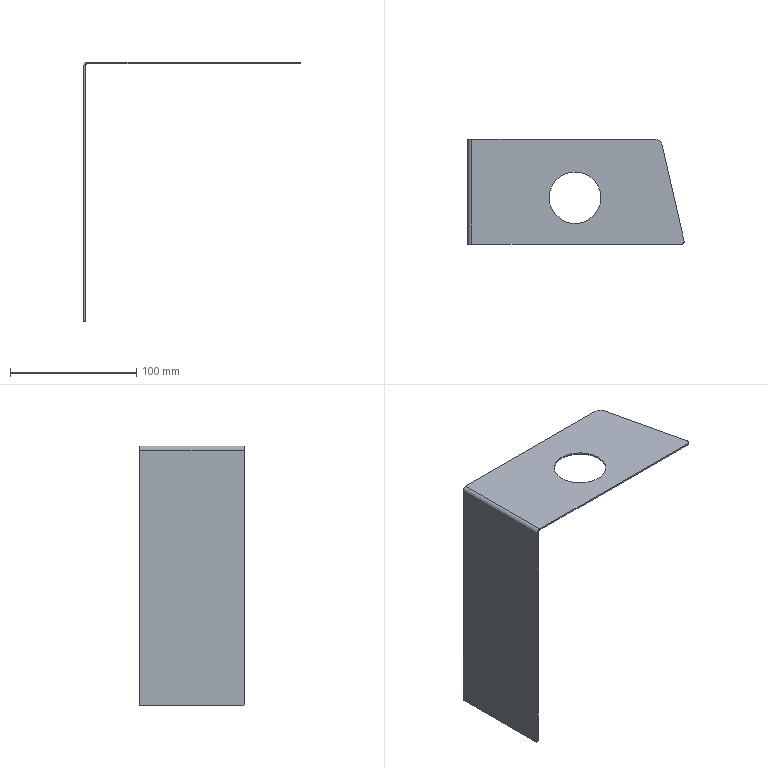Part | SolidWorks | features Fillet 2, FlatPattern 1, ICE 1, SMBaseFlange 1, SheetMetal 1 | 1 solid | 20 faces | box 171.49 x 83 x 206 mm | volume 34881 mm3 | plane 12 | cylinder 8 | commonest cylinder face diameters 4 x4 41 x2 6.4 x1 10 x1
STEP:
#1=CARTESIAN_POINT('',(171.49,2.,204.8));
#2=VERTEX_POINT('',#1);
#3=CARTESIAN_POINT('',(169.49,0.,204.8));
#4=VERTEX_POINT('',#3);
#5=CARTESIAN_POINT('',(169.49,2.,204.8));
#6=DIRECTION('',(0.,0.,-1.));
#7=DIRECTION('',(-1.,0.,0.));
#8=AXIS2_PLACEMENT_3D('',#5,#6,#7);
#9=CIRCLE('',#8,2.);
#10=EDGE_CURVE('',#2,#4,#9,.T.);
#11=ORIENTED_EDGE('',*,*,#10,.F.);
#12=CARTESIAN_POINT('',(171.49,2.,206.));
#13=VERTEX_POINT('',#12);
#14=CARTESIAN_POINT('',(171.49,2.,202.8));
#15=DIRECTION('',(0.,0.,1.));
#16=VECTOR('',#15,1000.);
#17=LINE('',#14,#16);
#18=EDGE_CURVE('',#2,#13,#17,.T.);
#19=ORIENTED_EDGE('',*,*,#18,.T.);
#20=CARTESIAN_POINT('',(169.49,0.,206.));
#21=VERTEX_POINT('',#20);
#22=CARTESIAN_POINT('',(169.49,2.,206.));
#23=DIRECTION('',(0.,0.,1.));
#24=DIRECTION('',(-1.,0.,0.));
#25=AXIS2_PLACEMENT_3D('',#22,#23,#24);
#26=CIRCLE('',#25,2.);
#27=EDGE_CURVE('',#21,#13,#26,.T.);
#28=ORIENTED_EDGE('',*,*,#27,.F.);
#29=CARTESIAN_POINT('',(169.49,0.,202.8));
#30=DIRECTION('',(0.,0.,1.));
#31=VECTOR('',#30,1000.);
#32=LINE('',#29,#31);
#33=EDGE_CURVE('',#4,#21,#32,.T.);
#34=ORIENTED_EDGE('',*,*,#33,.F.);
#35=EDGE_LOOP('',(#11,#19,#28,#34));
#36=FACE_OUTER_BOUND('',#35,.T.);
#37=CARTESIAN_POINT('',(169.49,2.,202.8));
#38=DIRECTION('',(0.,0.,1.));
#39=DIRECTION('',(1.,0.,0.));
#40=AXIS2_PLACEMENT_3D('',#37,#38,#39);
#41=CYLINDRICAL_SURFACE('',#40,2.);
#42=ADVANCED_FACE('',(#36),#41,.T.);
#43=CARTESIAN_POINT('',(64.5,36.8,206.));
#44=VERTEX_POINT('',#43);
#45=CARTESIAN_POINT('',(105.5,36.8,206.));
#46=VERTEX_POINT('',#45);
#47=CARTESIAN_POINT('',(85.,36.8,206.));
#48=DIRECTION('',(0.,0.,1.));
#49=DIRECTION('',(-1.,0.,0.));
#50=AXIS2_PLACEMENT_3D('',#47,#48,#49);
#51=CIRCLE('',#50,20.5);
#52=EDGE_CURVE('',#44,#46,#51,.T.);
#53=ORIENTED_EDGE('',*,*,#52,.T.);
#54=CARTESIAN_POINT('',(105.5,36.8,204.8));
#55=VERTEX_POINT('',#54);
#56=CARTESIAN_POINT('',(105.5,36.8,204.8));
#57=DIRECTION('',(0.,0.,-1.));
#58=VECTOR('',#57,1000.);
#59=LINE('',#56,#58);
#60=EDGE_CURVE('',#46,#55,#59,.T.);
#61=ORIENTED_EDGE('',*,*,#60,.T.);
#62=CARTESIAN_POINT('',(64.5,36.8,204.8));
#63=VERTEX_POINT('',#62);
#64=CARTESIAN_POINT('',(85.,36.8,204.8));
#65=DIRECTION('',(0.,0.,1.));
#66=DIRECTION('',(-1.,0.,0.));
#67=AXIS2_PLACEMENT_3D('',#64,#65,#66);
#68=CIRCLE('',#67,20.5);
#69=EDGE_CURVE('',#63,#55,#68,.T.);
#70=ORIENTED_EDGE('',*,*,#69,.F.);
#71=CARTESIAN_POINT('',(64.5,36.8,204.8));
#72=DIRECTION('',(0.,0.,-1.));
#73=VECTOR('',#72,1000.);
#74=LINE('',#71,#73);
#75=EDGE_CURVE('',#44,#63,#74,.T.);
#76=ORIENTED_EDGE('',*,*,#75,.F.);
#77=EDGE_LOOP('',(#53,#61,#70,#76));
#78=FACE_OUTER_BOUND('',#77,.T.);
#79=CARTESIAN_POINT('',(85.,36.8,204.8));
#80=DIRECTION('',(0.,0.,-1.));
#81=DIRECTION('',(-1.,0.,0.));
#82=AXIS2_PLACEMENT_3D('',#79,#80,#81);
#83=CYLINDRICAL_SURFACE('',#82,20.5);
#84=ADVANCED_FACE('',(#78),#83,.F.);
#85=CARTESIAN_POINT('',(3.2,0.,206.));
#86=VERTEX_POINT('',#85);
#87=CARTESIAN_POINT('',(0.,0.,206.));
#88=DIRECTION('',(1.,0.,0.));
#89=VECTOR('',#88,1000.);
#90=LINE('',#87,#89);
#91=EDGE_CURVE('',#86,#21,#90,.T.);
#92=ORIENTED_EDGE('',*,*,#91,.T.);
#93=ORIENTED_EDGE('',*,*,#27,.T.);
#94=CARTESIAN_POINT('',(171.44,2.446,206.));
#95=VERTEX_POINT('',#94);
#96=CARTESIAN_POINT('',(169.49,2.,206.));
#97=DIRECTION('',(0.,0.,1.));
#98=DIRECTION('',(-1.,0.,0.));
#99=AXIS2_PLACEMENT_3D('',#96,#97,#98);
#100=CIRCLE('',#99,2.);
#101=EDGE_CURVE('',#13,#95,#100,.T.);
#102=ORIENTED_EDGE('',*,*,#101,.T.);
#103=CARTESIAN_POINT('',(153.889,79.116,206.));
#104=VERTEX_POINT('',#103);
#105=CARTESIAN_POINT('',(153.,83.,206.));
#106=DIRECTION('',(0.2231,-0.9748,0.));
#107=VECTOR('',#106,1000.);
#108=LINE('',#105,#107);
#109=EDGE_CURVE('',#104,#95,#108,.T.);
#110=ORIENTED_EDGE('',*,*,#109,.F.);
#111=CARTESIAN_POINT('',(149.015,83.,206.));
#112=VERTEX_POINT('',#111);
#113=CARTESIAN_POINT('',(149.015,78.,206.));
#114=DIRECTION('',(0.,0.,1.));
#115=DIRECTION('',(-1.,0.,0.));
#116=AXIS2_PLACEMENT_3D('',#113,#114,#115);
#117=CIRCLE('',#116,5.);
#118=EDGE_CURVE('',#104,#112,#117,.T.);
#119=ORIENTED_EDGE('',*,*,#118,.T.);
#120=CARTESIAN_POINT('',(3.2,83.,206.));
#121=VERTEX_POINT('',#120);
#122=CARTESIAN_POINT('',(0.,83.,206.));
#123=DIRECTION('',(1.,0.,0.));
#124=VECTOR('',#123,1000.);
#125=LINE('',#122,#124);
#126=EDGE_CURVE('',#121,#112,#125,.T.);
#127=ORIENTED_EDGE('',*,*,#126,.F.);
#128=CARTESIAN_POINT('',(3.2,83.,206.));
#129=DIRECTION('',(0.,-1.,0.));
#130=VECTOR('',#129,1000.);
#131=LINE('',#128,#130);
#132=EDGE_CURVE('',#121,#86,#131,.T.);
#133=ORIENTED_EDGE('',*,*,#132,.T.);
#134=EDGE_LOOP('',(#92,#93,#102,#110,#119,#127,#133));
#135=FACE_OUTER_BOUND('',#134,.T.);
#136=ORIENTED_EDGE('',*,*,#52,.F.);
#137=CARTESIAN_POINT('',(85.,36.8,206.));
#138=DIRECTION('',(0.,0.,1.));
#139=DIRECTION('',(-1.,0.,0.));
#140=AXIS2_PLACEMENT_3D('',#137,#138,#139);
#141=CIRCLE('',#140,20.5);
#142=EDGE_CURVE('',#46,#44,#141,.T.);
#143=ORIENTED_EDGE('',*,*,#142,.F.);
#144=EDGE_LOOP('',(#136,#143));
#145=FACE_BOUND('',#144,.T.);
#146=CARTESIAN_POINT('',(0.,83.,206.));
#147=DIRECTION('',(0.,0.,-1.));
#148=DIRECTION('',(-1.,0.,0.));
#149=AXIS2_PLACEMENT_3D('',#146,#147,#148);
#150=PLANE('',#149);
#151=ADVANCED_FACE('',(#135,#145),#150,.F.);
#152=CARTESIAN_POINT('',(153.889,79.116,204.8));
#153=VERTEX_POINT('',#152);
#154=CARTESIAN_POINT('',(171.44,2.446,204.8));
#155=VERTEX_POINT('',#154);
#156=CARTESIAN_POINT('',(153.,83.,204.8));
#157=DIRECTION('',(0.2231,-0.9748,0.));
#158=VECTOR('',#157,1000.);
#159=LINE('',#156,#158);
#160=EDGE_CURVE('',#153,#155,#159,.T.);
#161=ORIENTED_EDGE('',*,*,#160,.T.);
#162=CARTESIAN_POINT('',(169.49,2.,204.8));
#163=DIRECTION('',(0.,0.,-1.));
#164=DIRECTION('',(-1.,0.,0.));
#165=AXIS2_PLACEMENT_3D('',#162,#163,#164);
#166=CIRCLE('',#165,2.);
#167=EDGE_CURVE('',#155,#2,#166,.T.);
#168=ORIENTED_EDGE('',*,*,#167,.T.);
#169=ORIENTED_EDGE('',*,*,#10,.T.);
#170=CARTESIAN_POINT('',(3.2,0.,204.8));
#171=VERTEX_POINT('',#170);
#172=CARTESIAN_POINT('',(0.,0.,204.8));
#173=DIRECTION('',(1.,0.,0.));
#174=VECTOR('',#173,1000.);
#175=LINE('',#172,#174);
#176=EDGE_CURVE('',#171,#4,#175,.T.);
#177=ORIENTED_EDGE('',*,*,#176,.F.);
#178=CARTESIAN_POINT('',(3.2,83.,204.8));
#179=VERTEX_POINT('',#178);
#180=CARTESIAN_POINT('',(3.2,83.,204.8));
#181=DIRECTION('',(0.,-1.,0.));
#182=VECTOR('',#181,1000.);
#183=LINE('',#180,#182);
#184=EDGE_CURVE('',#179,#171,#183,.T.);
#185=ORIENTED_EDGE('',*,*,#184,.F.);
#186=CARTESIAN_POINT('',(149.015,83.,204.8));
#187=VERTEX_POINT('',#186);
#188=CARTESIAN_POINT('',(0.,83.,204.8));
#189=DIRECTION('',(1.,0.,0.));
#190=VECTOR('',#189,1000.);
#191=LINE('',#188,#190);
#192=EDGE_CURVE('',#179,#187,#191,.T.);
#193=ORIENTED_EDGE('',*,*,#192,.T.);
#194=CARTESIAN_POINT('',(149.015,78.,204.8));
#195=DIRECTION('',(0.,0.,-1.));
#196=DIRECTION('',(-1.,0.,0.));
#197=AXIS2_PLACEMENT_3D('',#194,#195,#196);
#198=CIRCLE('',#197,5.);
#199=EDGE_CURVE('',#187,#153,#198,.T.);
#200=ORIENTED_EDGE('',*,*,#199,.T.);
#201=EDGE_LOOP('',(#161,#168,#169,#177,#185,#193,#200));
#202=FACE_OUTER_BOUND('',#201,.T.);
#203=ORIENTED_EDGE('',*,*,#69,.T.);
#204=CARTESIAN_POINT('',(85.,36.8,204.8));
#205=DIRECTION('',(0.,0.,1.));
#206=DIRECTION('',(-1.,0.,0.));
#207=AXIS2_PLACEMENT_3D('',#204,#205,#206);
#208=CIRCLE('',#207,20.5);
#209=EDGE_CURVE('',#55,#63,#208,.T.);
#210=ORIENTED_EDGE('',*,*,#209,.T.);
#211=EDGE_LOOP('',(#203,#210));
#212=FACE_BOUND('',#211,.T.);
#213=CARTESIAN_POINT('',(0.,83.,204.8));
#214=DIRECTION('',(0.,0.,-1.));
#215=DIRECTION('',(-1.,0.,0.));
#216=AXIS2_PLACEMENT_3D('',#213,#214,#215);
#217=PLANE('',#216);
#218=ADVANCED_FACE('',(#202,#212),#217,.T.);
#219=ORIENTED_EDGE('',*,*,#126,.T.);
#220=CARTESIAN_POINT('',(149.015,83.,202.8));
#221=DIRECTION('',(0.,0.,-1.));
#222=VECTOR('',#221,1000.);
#223=LINE('',#220,#222);
#224=EDGE_CURVE('',#112,#187,#223,.T.);
#225=ORIENTED_EDGE('',*,*,#224,.T.);
#226=ORIENTED_EDGE('',*,*,#192,.F.);
#227=CARTESIAN_POINT('',(3.2,83.,204.8));
#228=DIRECTION('',(0.,0.,1.));
#229=VECTOR('',#228,1000.);
#230=LINE('',#227,#229);
#231=EDGE_CURVE('',#179,#121,#230,.T.);
#232=ORIENTED_EDGE('',*,*,#231,.T.);
#233=EDGE_LOOP('',(#219,#225,#226,#232));
#234=FACE_OUTER_BOUND('',#233,.T.);
#235=CARTESIAN_POINT('',(3.2,83.,202.8));
#236=DIRECTION('',(0.,1.,0.));
#237=DIRECTION('',(1.,0.,0.));
#238=AXIS2_PLACEMENT_3D('',#235,#236,#237);
#239=PLANE('',#238);
#240=ADVANCED_FACE('',(#234),#239,.T.);
#241=CARTESIAN_POINT('',(0.,83.,202.8));
#242=VERTEX_POINT('',#241);
#243=CARTESIAN_POINT('',(1.2,83.,202.8));
#244=VERTEX_POINT('',#243);
#245=CARTESIAN_POINT('',(0.,83.,202.8));
#246=DIRECTION('',(1.,0.,0.));
#247=VECTOR('',#246,1000.);
#248=LINE('',#245,#247);
#249=EDGE_CURVE('',#242,#244,#248,.T.);
#250=ORIENTED_EDGE('',*,*,#249,.F.);
#251=CARTESIAN_POINT('',(3.2,83.,202.8));
#252=DIRECTION('',(0.,1.,0.));
#253=DIRECTION('',(0.,0.,-1.));
#254=AXIS2_PLACEMENT_3D('',#251,#252,#253);
#255=CIRCLE('',#254,3.2);
#256=EDGE_CURVE('',#242,#121,#255,.T.);
#257=ORIENTED_EDGE('',*,*,#256,.T.);
#258=ORIENTED_EDGE('',*,*,#231,.F.);
#259=CARTESIAN_POINT('',(3.2,83.,202.8));
#260=DIRECTION('',(0.,1.,0.));
#261=DIRECTION('',(1.,0.,0.));
#262=AXIS2_PLACEMENT_3D('',#259,#260,#261);
#263=CIRCLE('',#262,2.);
#264=EDGE_CURVE('',#244,#179,#263,.T.);
#265=ORIENTED_EDGE('',*,*,#264,.F.);
#266=EDGE_LOOP('',(#250,#257,#258,#265));
#267=FACE_OUTER_BOUND('',#266,.T.);
#268=CARTESIAN_POINT('',(0.,83.,202.8));
#269=DIRECTION('',(0.,1.,0.));
#270=DIRECTION('',(0.,0.,1.));
#271=AXIS2_PLACEMENT_3D('',#268,#269,#270);
#272=PLANE('',#271);
#273=ADVANCED_FACE('',(#267),#272,.T.);
#274=CARTESIAN_POINT('',(0.,83.,0.));
#275=VERTEX_POINT('',#274);
#276=CARTESIAN_POINT('',(0.,83.,0.));
#277=DIRECTION('',(0.,0.,1.));
#278=VECTOR('',#277,1000.);
#279=LINE('',#276,#278);
#280=EDGE_CURVE('',#275,#242,#279,.T.);
#281=ORIENTED_EDGE('',*,*,#280,.T.);
#282=ORIENTED_EDGE('',*,*,#249,.T.);
#283=CARTESIAN_POINT('',(1.2,83.,0.));
#284=VERTEX_POINT('',#283);
#285=CARTESIAN_POINT('',(1.2,83.,0.));
#286=DIRECTION('',(0.,0.,1.));
#287=VECTOR('',#286,1000.);
#288=LINE('',#285,#287);
#289=EDGE_CURVE('',#284,#244,#288,.T.);
#290=ORIENTED_EDGE('',*,*,#289,.F.);
#291=CARTESIAN_POINT('',(0.,83.,0.));
#292=DIRECTION('',(1.,0.,0.));
#293=VECTOR('',#292,1000.);
#294=LINE('',#291,#293);
#295=EDGE_CURVE('',#275,#284,#294,.T.);
#296=ORIENTED_EDGE('',*,*,#295,.F.);
#297=EDGE_LOOP('',(#281,#282,#290,#296));
#298=FACE_OUTER_BOUND('',#297,.T.);
#299=CARTESIAN_POINT('',(3.2,83.,204.8));
#300=DIRECTION('',(0.,1.,0.));
#301=DIRECTION('',(0.,0.,1.));
#302=AXIS2_PLACEMENT_3D('',#299,#300,#301);
#303=PLANE('',#302);
#304=ADVANCED_FACE('',(#298),#303,.T.);
#305=CARTESIAN_POINT('',(3.2,0.,206.));
#306=DIRECTION('',(0.,0.,-1.));
#307=VECTOR('',#306,1000.);
#308=LINE('',#305,#307);
#309=EDGE_CURVE('',#86,#171,#308,.T.);
#310=ORIENTED_EDGE('',*,*,#309,.F.);
#311=CARTESIAN_POINT('',(0.,0.,202.8));
#312=VERTEX_POINT('',#311);
#313=CARTESIAN_POINT('',(3.2,0.,202.8));
#314=DIRECTION('',(0.,1.,0.));
#315=DIRECTION('',(0.,0.,-1.));
#316=AXIS2_PLACEMENT_3D('',#313,#314,#315);
#317=CIRCLE('',#316,3.2);
#318=EDGE_CURVE('',#312,#86,#317,.T.);
#319=ORIENTED_EDGE('',*,*,#318,.F.);
#320=CARTESIAN_POINT('',(1.2,0.,202.8));
#321=VERTEX_POINT('',#320);
#322=CARTESIAN_POINT('',(1.2,0.,202.8));
#323=DIRECTION('',(-1.,0.,0.));
#324=VECTOR('',#323,1000.);
#325=LINE('',#322,#324);
#326=EDGE_CURVE('',#321,#312,#325,.T.);
#327=ORIENTED_EDGE('',*,*,#326,.F.);
#328=CARTESIAN_POINT('',(3.2,0.,202.8));
#329=DIRECTION('',(0.,1.,0.));
#330=DIRECTION('',(1.,0.,0.));
#331=AXIS2_PLACEMENT_3D('',#328,#329,#330);
#332=CIRCLE('',#331,2.);
#333=EDGE_CURVE('',#321,#171,#332,.T.);
#334=ORIENTED_EDGE('',*,*,#333,.T.);
#335=EDGE_LOOP('',(#310,#319,#327,#334));
#336=FACE_OUTER_BOUND('',#335,.T.);
#337=CARTESIAN_POINT('',(3.2,0.,206.));
#338=DIRECTION('',(0.,-1.,0.));
#339=DIRECTION('',(0.,0.,-1.));
#340=AXIS2_PLACEMENT_3D('',#337,#338,#339);
#341=PLANE('',#340);
#342=ADVANCED_FACE('',(#336),#341,.T.);
#343=ORIENTED_EDGE('',*,*,#176,.T.);
#344=ORIENTED_EDGE('',*,*,#33,.T.);
#345=ORIENTED_EDGE('',*,*,#91,.F.);
#346=ORIENTED_EDGE('',*,*,#309,.T.);
#347=EDGE_LOOP('',(#343,#344,#345,#346));
#348=FACE_OUTER_BOUND('',#347,.T.);
#349=CARTESIAN_POINT('',(1.2,0.,202.8));
#350=DIRECTION('',(0.,-1.,0.));
#351=DIRECTION('',(0.,0.,-1.));
#352=AXIS2_PLACEMENT_3D('',#349,#350,#351);
#353=PLANE('',#352);
#354=ADVANCED_FACE('',(#348),#353,.T.);
#355=ORIENTED_EDGE('',*,*,#333,.F.);
#356=CARTESIAN_POINT('',(1.2,83.,202.8));
#357=DIRECTION('',(0.,-1.,0.));
#358=VECTOR('',#357,1000.);
#359=LINE('',#356,#358);
#360=EDGE_CURVE('',#244,#321,#359,.T.);
#361=ORIENTED_EDGE('',*,*,#360,.F.);
#362=ORIENTED_EDGE('',*,*,#264,.T.);
#363=ORIENTED_EDGE('',*,*,#184,.T.);
#364=EDGE_LOOP('',(#355,#361,#362,#363));
#365=FACE_OUTER_BOUND('',#364,.T.);
#366=CARTESIAN_POINT('',(3.2,83.,202.8));
#367=DIRECTION('',(0.,-1.,0.));
#368=DIRECTION('',(0.,0.,-1.));
#369=AXIS2_PLACEMENT_3D('',#366,#367,#368);
#370=CYLINDRICAL_SURFACE('',#369,2.);
#371=ADVANCED_FACE('',(#365),#370,.F.);
#372=CARTESIAN_POINT('',(1.2,0.,2.));
#373=VERTEX_POINT('',#372);
#374=CARTESIAN_POINT('',(1.2,0.,0.));
#375=DIRECTION('',(0.,0.,1.));
#376=VECTOR('',#375,1000.);
#377=LINE('',#374,#376);
#378=EDGE_CURVE('',#373,#321,#377,.T.);
#379=ORIENTED_EDGE('',*,*,#378,.F.);
#380=CARTESIAN_POINT('',(1.2,2.,0.));
#381=VERTEX_POINT('',#380);
#382=CARTESIAN_POINT('',(1.2,2.,2.));
#383=DIRECTION('',(1.,0.,0.));
#384=DIRECTION('',(0.,0.,-1.));
#385=AXIS2_PLACEMENT_3D('',#382,#383,#384);
#386=CIRCLE('',#385,2.);
#387=EDGE_CURVE('',#373,#381,#386,.T.);
#388=ORIENTED_EDGE('',*,*,#387,.T.);
#389=CARTESIAN_POINT('',(1.2,83.,0.));
#390=DIRECTION('',(0.,-1.,0.));
#391=VECTOR('',#390,1000.);
#392=LINE('',#389,#391);
#393=EDGE_CURVE('',#284,#381,#392,.T.);
#394=ORIENTED_EDGE('',*,*,#393,.F.);
#395=ORIENTED_EDGE('',*,*,#289,.T.);
#396=ORIENTED_EDGE('',*,*,#360,.T.);
#397=EDGE_LOOP('',(#379,#388,#394,#395,#396));
#398=FACE_OUTER_BOUND('',#397,.T.);
#399=CARTESIAN_POINT('',(1.2,83.,0.));
#400=DIRECTION('',(1.,0.,0.));
#401=DIRECTION('',(0.,0.,-1.));
#402=AXIS2_PLACEMENT_3D('',#399,#400,#401);
#403=PLANE('',#402);
#404=ADVANCED_FACE('',(#398),#403,.T.);
#405=ORIENTED_EDGE('',*,*,#393,.T.);
#406=CARTESIAN_POINT('',(0.,2.,0.));
#407=VERTEX_POINT('',#406);
#408=CARTESIAN_POINT('',(0.,2.,0.));
#409=DIRECTION('',(-1.,0.,0.));
#410=VECTOR('',#409,1000.);
#411=LINE('',#408,#410);
#412=EDGE_CURVE('',#381,#407,#411,.T.);
#413=ORIENTED_EDGE('',*,*,#412,.T.);
#414=CARTESIAN_POINT('',(0.,83.,0.));
#415=DIRECTION('',(0.,-1.,0.));
#416=VECTOR('',#415,1000.);
#417=LINE('',#414,#416);
#418=EDGE_CURVE('',#275,#407,#417,.T.);
#419=ORIENTED_EDGE('',*,*,#418,.F.);
#420=ORIENTED_EDGE('',*,*,#295,.T.);
#421=EDGE_LOOP('',(#405,#413,#419,#420));
#422=FACE_OUTER_BOUND('',#421,.T.);
#423=CARTESIAN_POINT('',(0.,83.,0.));
#424=DIRECTION('',(0.,0.,-1.));
#425=DIRECTION('',(-1.,0.,0.));
#426=AXIS2_PLACEMENT_3D('',#423,#424,#425);
#427=PLANE('',#426);
#428=ADVANCED_FACE('',(#422),#427,.T.);
#429=ORIENTED_EDGE('',*,*,#418,.T.);
#430=CARTESIAN_POINT('',(0.,0.,2.));
#431=VERTEX_POINT('',#430);
#432=CARTESIAN_POINT('',(0.,2.,2.));
#433=DIRECTION('',(-1.,0.,0.));
#434=DIRECTION('',(0.,0.,-1.));
#435=AXIS2_PLACEMENT_3D('',#432,#433,#434);
#436=CIRCLE('',#435,2.);
#437=EDGE_CURVE('',#407,#431,#436,.T.);
#438=ORIENTED_EDGE('',*,*,#437,.T.);
#439=CARTESIAN_POINT('',(0.,0.,0.));
#440=DIRECTION('',(0.,0.,1.));
#441=VECTOR('',#440,1000.);
#442=LINE('',#439,#441);
#443=EDGE_CURVE('',#431,#312,#442,.T.);
#444=ORIENTED_EDGE('',*,*,#443,.T.);
#445=CARTESIAN_POINT('',(0.,83.,202.8));
#446=DIRECTION('',(0.,-1.,0.));
#447=VECTOR('',#446,1000.);
#448=LINE('',#445,#447);
#449=EDGE_CURVE('',#242,#312,#448,.T.);
#450=ORIENTED_EDGE('',*,*,#449,.F.);
#451=ORIENTED_EDGE('',*,*,#280,.F.);
#452=EDGE_LOOP('',(#429,#438,#444,#450,#451));
#453=FACE_OUTER_BOUND('',#452,.T.);
#454=CARTESIAN_POINT('',(0.,83.,0.));
#455=DIRECTION('',(1.,0.,0.));
#456=DIRECTION('',(0.,0.,-1.));
#457=AXIS2_PLACEMENT_3D('',#454,#455,#456);
#458=PLANE('',#457);
#459=ADVANCED_FACE('',(#453),#458,.F.);
#460=ORIENTED_EDGE('',*,*,#318,.T.);
#461=ORIENTED_EDGE('',*,*,#132,.F.);
#462=ORIENTED_EDGE('',*,*,#256,.F.);
#463=ORIENTED_EDGE('',*,*,#449,.T.);
#464=EDGE_LOOP('',(#460,#461,#462,#463));
#465=FACE_OUTER_BOUND('',#464,.T.);
#466=CARTESIAN_POINT('',(3.2,83.,202.8));
#467=DIRECTION('',(0.,-1.,0.));
#468=DIRECTION('',(0.,0.,-1.));
#469=AXIS2_PLACEMENT_3D('',#466,#467,#468);
#470=CYLINDRICAL_SURFACE('',#469,3.2);
#471=ADVANCED_FACE('',(#465),#470,.T.);
#472=ORIENTED_EDGE('',*,*,#443,.F.);
#473=CARTESIAN_POINT('',(1.2,0.,2.));
#474=DIRECTION('',(1.,0.,0.));
#475=VECTOR('',#474,1000.);
#476=LINE('',#473,#475);
#477=EDGE_CURVE('',#431,#373,#476,.T.);
#478=ORIENTED_EDGE('',*,*,#477,.T.);
#479=ORIENTED_EDGE('',*,*,#378,.T.);
#480=ORIENTED_EDGE('',*,*,#326,.T.);
#481=EDGE_LOOP('',(#472,#478,#479,#480));
#482=FACE_OUTER_BOUND('',#481,.T.);
#483=CARTESIAN_POINT('',(3.2,0.,202.8));
#484=DIRECTION('',(0.,1.,0.));
#485=DIRECTION('',(1.,0.,0.));
#486=AXIS2_PLACEMENT_3D('',#483,#484,#485);
#487=PLANE('',#486);
#488=ADVANCED_FACE('',(#482),#487,.F.);
#489=ORIENTED_EDGE('',*,*,#109,.T.);
#490=CARTESIAN_POINT('',(171.44,2.446,204.8));
#491=DIRECTION('',(0.,0.,-1.));
#492=VECTOR('',#491,1000.);
#493=LINE('',#490,#492);
#494=EDGE_CURVE('',#95,#155,#493,.T.);
#495=ORIENTED_EDGE('',*,*,#494,.T.);
#496=ORIENTED_EDGE('',*,*,#160,.F.);
#497=CARTESIAN_POINT('',(153.889,79.116,204.8));
#498=DIRECTION('',(0.,0.,1.));
#499=VECTOR('',#498,1000.);
#500=LINE('',#497,#499);
#501=EDGE_CURVE('',#153,#104,#500,.T.);
#502=ORIENTED_EDGE('',*,*,#501,.T.);
#503=EDGE_LOOP('',(#489,#495,#496,#502));
#504=FACE_OUTER_BOUND('',#503,.T.);
#505=CARTESIAN_POINT('',(153.,83.,204.8));
#506=DIRECTION('',(0.9748,0.2231,0.));
#507=DIRECTION('',(0.2231,-0.9748,0.));
#508=AXIS2_PLACEMENT_3D('',#505,#506,#507);
#509=PLANE('',#508);
#510=ADVANCED_FACE('',(#504),#509,.T.);
#511=ORIENTED_EDGE('',*,*,#60,.F.);
#512=ORIENTED_EDGE('',*,*,#142,.T.);
#513=ORIENTED_EDGE('',*,*,#75,.T.);
#514=ORIENTED_EDGE('',*,*,#209,.F.);
#515=EDGE_LOOP('',(#511,#512,#513,#514));
#516=FACE_OUTER_BOUND('',#515,.T.);
#517=CARTESIAN_POINT('',(85.,36.8,204.8));
#518=DIRECTION('',(0.,0.,-1.));
#519=DIRECTION('',(-1.,0.,0.));
#520=AXIS2_PLACEMENT_3D('',#517,#518,#519);
#521=CYLINDRICAL_SURFACE('',#520,20.5);
#522=ADVANCED_FACE('',(#516),#521,.F.);
#523=ORIENTED_EDGE('',*,*,#199,.F.);
#524=ORIENTED_EDGE('',*,*,#224,.F.);
#525=ORIENTED_EDGE('',*,*,#118,.F.);
#526=ORIENTED_EDGE('',*,*,#501,.F.);
#527=EDGE_LOOP('',(#523,#524,#525,#526));
#528=FACE_OUTER_BOUND('',#527,.T.);
#529=CARTESIAN_POINT('',(149.015,78.,204.8));
#530=DIRECTION('',(0.,0.,1.));
#531=DIRECTION('',(1.,0.,0.));
#532=AXIS2_PLACEMENT_3D('',#529,#530,#531);
#533=CYLINDRICAL_SURFACE('',#532,5.);
#534=ADVANCED_FACE('',(#528),#533,.T.);
#535=ORIENTED_EDGE('',*,*,#437,.F.);
#536=ORIENTED_EDGE('',*,*,#412,.F.);
#537=ORIENTED_EDGE('',*,*,#387,.F.);
#538=ORIENTED_EDGE('',*,*,#477,.F.);
#539=EDGE_LOOP('',(#535,#536,#537,#538));
#540=FACE_OUTER_BOUND('',#539,.T.);
#541=CARTESIAN_POINT('',(3.2,2.,2.));
#542=DIRECTION('',(-1.,0.,0.));
#543=DIRECTION('',(0.,0.,1.));
#544=AXIS2_PLACEMENT_3D('',#541,#542,#543);
#545=CYLINDRICAL_SURFACE('',#544,2.);
#546=ADVANCED_FACE('',(#540),#545,.T.);
#547=ORIENTED_EDGE('',*,*,#18,.F.);
#548=ORIENTED_EDGE('',*,*,#167,.F.);
#549=ORIENTED_EDGE('',*,*,#494,.F.);
#550=ORIENTED_EDGE('',*,*,#101,.F.);
#551=EDGE_LOOP('',(#547,#548,#549,#550));
#552=FACE_OUTER_BOUND('',#551,.T.);
#553=CARTESIAN_POINT('',(169.49,2.,202.8));
#554=DIRECTION('',(0.,0.,1.));
#555=DIRECTION('',(1.,0.,0.));
#556=AXIS2_PLACEMENT_3D('',#553,#554,#555);
#557=CYLINDRICAL_SURFACE('',#556,2.);
#558=ADVANCED_FACE('',(#552),#557,.T.);
#559=CLOSED_SHELL('',(#42,#84,#151,#218,#240,#273,#304,#342,#354,#371,#404,#428,#459,#471,#488,#510,#522,#534,#546,#558));
#560=MANIFOLD_SOLID_BREP('',#559);
#561=CARTESIAN_POINT('',(0.,0.,0.));
#562=DIRECTION('',(0.,0.,1.));
#563=DIRECTION('',(1.,0.,0.));
#564=AXIS2_PLACEMENT_3D('',#561,#562,#563);
#565=(LENGTH_UNIT()NAMED_UNIT(*)SI_UNIT(.MILLI.,.METRE.));
#566=UNCERTAINTY_MEASURE_WITH_UNIT(LENGTH_MEASURE(0.00001),#565,'','');
#567=(NAMED_UNIT(*)PLANE_ANGLE_UNIT()SI_UNIT($,.RADIAN.));
#568=(NAMED_UNIT(*)SI_UNIT($,.STERADIAN.)SOLID_ANGLE_UNIT());
#569=(GEOMETRIC_REPRESENTATION_CONTEXT(3)GLOBAL_UNCERTAINTY_ASSIGNED_CONTEXT((#566))GLOBAL_UNIT_ASSIGNED_CONTEXT((#565,#567,#568))REPRESENTATION_CONTEXT('',''));
#570=ADVANCED_BREP_SHAPE_REPRESENTATION('',(#560,#564),#569);